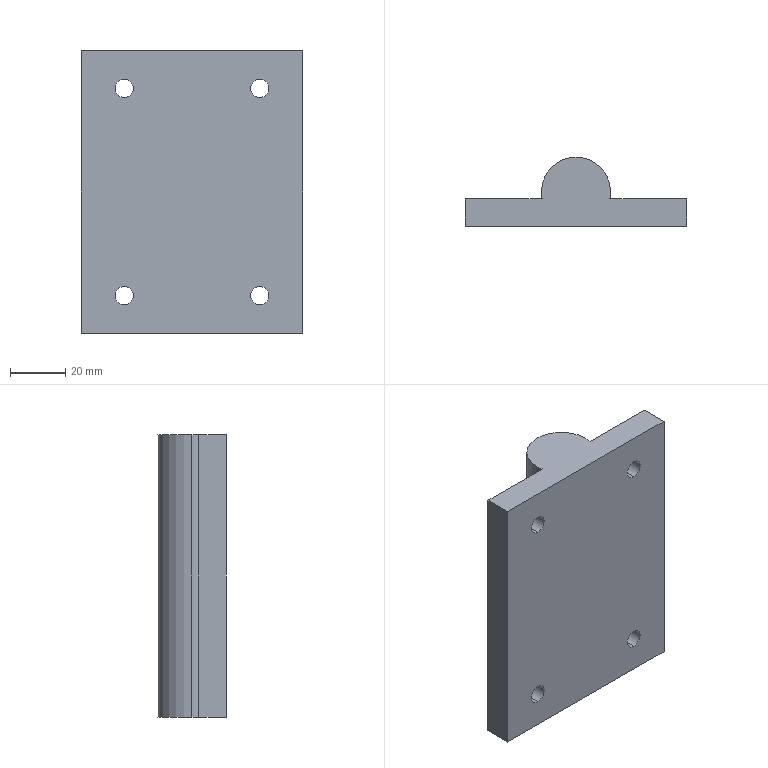Part | SolidWorks | features BaseBody 1 | 1 solid | 26 faces | box 80 x 25 x 102 mm | volume 111075 mm3 | cylinder 11 | cone 8 | plane 7 | commonest cylinder face diameters 6.6 x8 25 x3
STEP:
#1=CARTESIAN_POINT('',(-24.5,6.9,-40.8));
#2=VERTEX_POINT('',#1);
#3=CARTESIAN_POINT('',(-24.5,10.,-43.9));
#4=VERTEX_POINT('',#3);
#5=CARTESIAN_POINT('',(-24.5,10.,-43.9));
#6=DIRECTION('',(0.,0.7071,-0.7071));
#7=VECTOR('',#6,1000.);
#8=LINE('',#5,#7);
#9=EDGE_CURVE('',#2,#4,#8,.T.);
#10=ORIENTED_EDGE('',*,*,#9,.F.);
#11=CARTESIAN_POINT('',(-24.5,6.9,-34.2));
#12=VERTEX_POINT('',#11);
#13=CARTESIAN_POINT('',(-24.5,6.9,-37.5));
#14=DIRECTION('',(0.,1.,0.));
#15=DIRECTION('',(0.,0.,1.));
#16=AXIS2_PLACEMENT_3D('',#13,#14,#15);
#17=CIRCLE('',#16,3.3);
#18=EDGE_CURVE('',#12,#2,#17,.T.);
#19=ORIENTED_EDGE('',*,*,#18,.F.);
#20=CARTESIAN_POINT('',(-24.5,10.,-31.1));
#21=VERTEX_POINT('',#20);
#22=CARTESIAN_POINT('',(-24.5,10.,-31.1));
#23=DIRECTION('',(0.,0.7071,0.7071));
#24=VECTOR('',#23,1000.);
#25=LINE('',#22,#24);
#26=EDGE_CURVE('',#12,#21,#25,.T.);
#27=ORIENTED_EDGE('',*,*,#26,.T.);
#28=CARTESIAN_POINT('',(-24.5,10.,-37.5));
#29=DIRECTION('',(0.,1.,0.));
#30=DIRECTION('',(0.,0.,1.));
#31=AXIS2_PLACEMENT_3D('',#28,#29,#30);
#32=CIRCLE('',#31,6.4);
#33=EDGE_CURVE('',#21,#4,#32,.T.);
#34=ORIENTED_EDGE('',*,*,#33,.T.);
#35=EDGE_LOOP('',(#10,#19,#27,#34));
#36=FACE_OUTER_BOUND('',#35,.T.);
#37=CARTESIAN_POINT('',(-24.5,10.,-37.5));
#38=DIRECTION('',(0.,1.,0.));
#39=DIRECTION('',(0.,0.,1.));
#40=AXIS2_PLACEMENT_3D('',#37,#38,#39);
#41=CONICAL_SURFACE('',#40,6.4,0.7854);
#42=ADVANCED_FACE('',(#36),#41,.F.);
#43=CARTESIAN_POINT('',(-24.5,0.,-40.8));
#44=VERTEX_POINT('',#43);
#45=CARTESIAN_POINT('',(-24.5,10.,-40.8));
#46=DIRECTION('',(0.,1.,0.));
#47=VECTOR('',#46,1000.);
#48=LINE('',#45,#47);
#49=EDGE_CURVE('',#44,#2,#48,.T.);
#50=ORIENTED_EDGE('',*,*,#49,.F.);
#51=CARTESIAN_POINT('',(-24.5,0.,-34.2));
#52=VERTEX_POINT('',#51);
#53=CARTESIAN_POINT('',(-24.5,0.,-37.5));
#54=DIRECTION('',(0.,1.,0.));
#55=DIRECTION('',(0.,0.,1.));
#56=AXIS2_PLACEMENT_3D('',#53,#54,#55);
#57=CIRCLE('',#56,3.3);
#58=EDGE_CURVE('',#52,#44,#57,.T.);
#59=ORIENTED_EDGE('',*,*,#58,.F.);
#60=CARTESIAN_POINT('',(-24.5,10.,-34.2));
#61=DIRECTION('',(0.,1.,0.));
#62=VECTOR('',#61,1000.);
#63=LINE('',#60,#62);
#64=EDGE_CURVE('',#52,#12,#63,.T.);
#65=ORIENTED_EDGE('',*,*,#64,.T.);
#66=ORIENTED_EDGE('',*,*,#18,.T.);
#67=EDGE_LOOP('',(#50,#59,#65,#66));
#68=FACE_OUTER_BOUND('',#67,.T.);
#69=CARTESIAN_POINT('',(-24.5,10.,-37.5));
#70=DIRECTION('',(0.,1.,0.));
#71=DIRECTION('',(0.,0.,1.));
#72=AXIS2_PLACEMENT_3D('',#69,#70,#71);
#73=CYLINDRICAL_SURFACE('',#72,3.3);
#74=ADVANCED_FACE('',(#68),#73,.F.);
#75=CARTESIAN_POINT('',(-24.5,6.9,34.2));
#76=VERTEX_POINT('',#75);
#77=CARTESIAN_POINT('',(-24.5,10.,31.1));
#78=VERTEX_POINT('',#77);
#79=CARTESIAN_POINT('',(-24.5,10.,31.1));
#80=DIRECTION('',(0.,0.7071,-0.7071));
#81=VECTOR('',#80,1000.);
#82=LINE('',#79,#81);
#83=EDGE_CURVE('',#76,#78,#82,.T.);
#84=ORIENTED_EDGE('',*,*,#83,.F.);
#85=CARTESIAN_POINT('',(-24.5,6.9,40.8));
#86=VERTEX_POINT('',#85);
#87=CARTESIAN_POINT('',(-24.5,6.9,37.5));
#88=DIRECTION('',(0.,1.,0.));
#89=DIRECTION('',(0.,0.,1.));
#90=AXIS2_PLACEMENT_3D('',#87,#88,#89);
#91=CIRCLE('',#90,3.3);
#92=EDGE_CURVE('',#86,#76,#91,.T.);
#93=ORIENTED_EDGE('',*,*,#92,.F.);
#94=CARTESIAN_POINT('',(-24.5,10.,43.9));
#95=VERTEX_POINT('',#94);
#96=CARTESIAN_POINT('',(-24.5,10.,43.9));
#97=DIRECTION('',(0.,0.7071,0.7071));
#98=VECTOR('',#97,1000.);
#99=LINE('',#96,#98);
#100=EDGE_CURVE('',#86,#95,#99,.T.);
#101=ORIENTED_EDGE('',*,*,#100,.T.);
#102=CARTESIAN_POINT('',(-24.5,10.,37.5));
#103=DIRECTION('',(0.,1.,0.));
#104=DIRECTION('',(0.,0.,1.));
#105=AXIS2_PLACEMENT_3D('',#102,#103,#104);
#106=CIRCLE('',#105,6.4);
#107=EDGE_CURVE('',#95,#78,#106,.T.);
#108=ORIENTED_EDGE('',*,*,#107,.T.);
#109=EDGE_LOOP('',(#84,#93,#101,#108));
#110=FACE_OUTER_BOUND('',#109,.T.);
#111=CARTESIAN_POINT('',(-24.5,10.,37.5));
#112=DIRECTION('',(0.,1.,0.));
#113=DIRECTION('',(0.,0.,1.));
#114=AXIS2_PLACEMENT_3D('',#111,#112,#113);
#115=CONICAL_SURFACE('',#114,6.4,0.7854);
#116=ADVANCED_FACE('',(#110),#115,.F.);
#117=CARTESIAN_POINT('',(-24.5,0.,34.2));
#118=VERTEX_POINT('',#117);
#119=CARTESIAN_POINT('',(-24.5,10.,34.2));
#120=DIRECTION('',(0.,1.,0.));
#121=VECTOR('',#120,1000.);
#122=LINE('',#119,#121);
#123=EDGE_CURVE('',#118,#76,#122,.T.);
#124=ORIENTED_EDGE('',*,*,#123,.F.);
#125=CARTESIAN_POINT('',(-24.5,0.,40.8));
#126=VERTEX_POINT('',#125);
#127=CARTESIAN_POINT('',(-24.5,0.,37.5));
#128=DIRECTION('',(0.,1.,0.));
#129=DIRECTION('',(0.,0.,1.));
#130=AXIS2_PLACEMENT_3D('',#127,#128,#129);
#131=CIRCLE('',#130,3.3);
#132=EDGE_CURVE('',#126,#118,#131,.T.);
#133=ORIENTED_EDGE('',*,*,#132,.F.);
#134=CARTESIAN_POINT('',(-24.5,10.,40.8));
#135=DIRECTION('',(0.,1.,0.));
#136=VECTOR('',#135,1000.);
#137=LINE('',#134,#136);
#138=EDGE_CURVE('',#126,#86,#137,.T.);
#139=ORIENTED_EDGE('',*,*,#138,.T.);
#140=ORIENTED_EDGE('',*,*,#92,.T.);
#141=EDGE_LOOP('',(#124,#133,#139,#140));
#142=FACE_OUTER_BOUND('',#141,.T.);
#143=CARTESIAN_POINT('',(-24.5,10.,37.5));
#144=DIRECTION('',(0.,1.,0.));
#145=DIRECTION('',(0.,0.,1.));
#146=AXIS2_PLACEMENT_3D('',#143,#144,#145);
#147=CYLINDRICAL_SURFACE('',#146,3.3);
#148=ADVANCED_FACE('',(#142),#147,.F.);
#149=CARTESIAN_POINT('',(24.5,6.9,34.2));
#150=VERTEX_POINT('',#149);
#151=CARTESIAN_POINT('',(24.5,10.,31.1));
#152=VERTEX_POINT('',#151);
#153=CARTESIAN_POINT('',(24.5,10.,31.1));
#154=DIRECTION('',(0.,0.7071,-0.7071));
#155=VECTOR('',#154,1000.);
#156=LINE('',#153,#155);
#157=EDGE_CURVE('',#150,#152,#156,.T.);
#158=ORIENTED_EDGE('',*,*,#157,.F.);
#159=CARTESIAN_POINT('',(24.5,6.9,40.8));
#160=VERTEX_POINT('',#159);
#161=CARTESIAN_POINT('',(24.5,6.9,37.5));
#162=DIRECTION('',(0.,1.,0.));
#163=DIRECTION('',(0.,0.,1.));
#164=AXIS2_PLACEMENT_3D('',#161,#162,#163);
#165=CIRCLE('',#164,3.3);
#166=EDGE_CURVE('',#160,#150,#165,.T.);
#167=ORIENTED_EDGE('',*,*,#166,.F.);
#168=CARTESIAN_POINT('',(24.5,10.,43.9));
#169=VERTEX_POINT('',#168);
#170=CARTESIAN_POINT('',(24.5,10.,43.9));
#171=DIRECTION('',(0.,0.7071,0.7071));
#172=VECTOR('',#171,1000.);
#173=LINE('',#170,#172);
#174=EDGE_CURVE('',#160,#169,#173,.T.);
#175=ORIENTED_EDGE('',*,*,#174,.T.);
#176=CARTESIAN_POINT('',(24.5,10.,37.5));
#177=DIRECTION('',(0.,1.,0.));
#178=DIRECTION('',(0.,0.,1.));
#179=AXIS2_PLACEMENT_3D('',#176,#177,#178);
#180=CIRCLE('',#179,6.4);
#181=EDGE_CURVE('',#169,#152,#180,.T.);
#182=ORIENTED_EDGE('',*,*,#181,.T.);
#183=EDGE_LOOP('',(#158,#167,#175,#182));
#184=FACE_OUTER_BOUND('',#183,.T.);
#185=CARTESIAN_POINT('',(24.5,10.,37.5));
#186=DIRECTION('',(0.,1.,0.));
#187=DIRECTION('',(0.,0.,1.));
#188=AXIS2_PLACEMENT_3D('',#185,#186,#187);
#189=CONICAL_SURFACE('',#188,6.4,0.7854);
#190=ADVANCED_FACE('',(#184),#189,.F.);
#191=CARTESIAN_POINT('',(24.5,0.,34.2));
#192=VERTEX_POINT('',#191);
#193=CARTESIAN_POINT('',(24.5,10.,34.2));
#194=DIRECTION('',(0.,1.,0.));
#195=VECTOR('',#194,1000.);
#196=LINE('',#193,#195);
#197=EDGE_CURVE('',#192,#150,#196,.T.);
#198=ORIENTED_EDGE('',*,*,#197,.F.);
#199=CARTESIAN_POINT('',(24.5,0.,40.8));
#200=VERTEX_POINT('',#199);
#201=CARTESIAN_POINT('',(24.5,0.,37.5));
#202=DIRECTION('',(0.,1.,0.));
#203=DIRECTION('',(0.,0.,1.));
#204=AXIS2_PLACEMENT_3D('',#201,#202,#203);
#205=CIRCLE('',#204,3.3);
#206=EDGE_CURVE('',#200,#192,#205,.T.);
#207=ORIENTED_EDGE('',*,*,#206,.F.);
#208=CARTESIAN_POINT('',(24.5,10.,40.8));
#209=DIRECTION('',(0.,1.,0.));
#210=VECTOR('',#209,1000.);
#211=LINE('',#208,#210);
#212=EDGE_CURVE('',#200,#160,#211,.T.);
#213=ORIENTED_EDGE('',*,*,#212,.T.);
#214=ORIENTED_EDGE('',*,*,#166,.T.);
#215=EDGE_LOOP('',(#198,#207,#213,#214));
#216=FACE_OUTER_BOUND('',#215,.T.);
#217=CARTESIAN_POINT('',(24.5,10.,37.5));
#218=DIRECTION('',(0.,1.,0.));
#219=DIRECTION('',(0.,0.,1.));
#220=AXIS2_PLACEMENT_3D('',#217,#218,#219);
#221=CYLINDRICAL_SURFACE('',#220,3.3);
#222=ADVANCED_FACE('',(#216),#221,.F.);
#223=CARTESIAN_POINT('',(24.5,6.9,-40.8));
#224=VERTEX_POINT('',#223);
#225=CARTESIAN_POINT('',(24.5,10.,-43.9));
#226=VERTEX_POINT('',#225);
#227=CARTESIAN_POINT('',(24.5,10.,-43.9));
#228=DIRECTION('',(0.,0.7071,-0.7071));
#229=VECTOR('',#228,1000.);
#230=LINE('',#227,#229);
#231=EDGE_CURVE('',#224,#226,#230,.T.);
#232=ORIENTED_EDGE('',*,*,#231,.F.);
#233=CARTESIAN_POINT('',(24.5,6.9,-34.2));
#234=VERTEX_POINT('',#233);
#235=CARTESIAN_POINT('',(24.5,6.9,-37.5));
#236=DIRECTION('',(0.,1.,0.));
#237=DIRECTION('',(0.,0.,1.));
#238=AXIS2_PLACEMENT_3D('',#235,#236,#237);
#239=CIRCLE('',#238,3.3);
#240=EDGE_CURVE('',#234,#224,#239,.T.);
#241=ORIENTED_EDGE('',*,*,#240,.F.);
#242=CARTESIAN_POINT('',(24.5,10.,-31.1));
#243=VERTEX_POINT('',#242);
#244=CARTESIAN_POINT('',(24.5,10.,-31.1));
#245=DIRECTION('',(0.,0.7071,0.7071));
#246=VECTOR('',#245,1000.);
#247=LINE('',#244,#246);
#248=EDGE_CURVE('',#234,#243,#247,.T.);
#249=ORIENTED_EDGE('',*,*,#248,.T.);
#250=CARTESIAN_POINT('',(24.5,10.,-37.5));
#251=DIRECTION('',(0.,1.,0.));
#252=DIRECTION('',(0.,0.,1.));
#253=AXIS2_PLACEMENT_3D('',#250,#251,#252);
#254=CIRCLE('',#253,6.4);
#255=EDGE_CURVE('',#243,#226,#254,.T.);
#256=ORIENTED_EDGE('',*,*,#255,.T.);
#257=EDGE_LOOP('',(#232,#241,#249,#256));
#258=FACE_OUTER_BOUND('',#257,.T.);
#259=CARTESIAN_POINT('',(24.5,10.,-37.5));
#260=DIRECTION('',(0.,1.,0.));
#261=DIRECTION('',(0.,0.,1.));
#262=AXIS2_PLACEMENT_3D('',#259,#260,#261);
#263=CONICAL_SURFACE('',#262,6.4,0.7854);
#264=ADVANCED_FACE('',(#258),#263,.F.);
#265=CARTESIAN_POINT('',(24.5,0.,-40.8));
#266=VERTEX_POINT('',#265);
#267=CARTESIAN_POINT('',(24.5,10.,-40.8));
#268=DIRECTION('',(0.,1.,0.));
#269=VECTOR('',#268,1000.);
#270=LINE('',#267,#269);
#271=EDGE_CURVE('',#266,#224,#270,.T.);
#272=ORIENTED_EDGE('',*,*,#271,.F.);
#273=CARTESIAN_POINT('',(24.5,0.,-34.2));
#274=VERTEX_POINT('',#273);
#275=CARTESIAN_POINT('',(24.5,0.,-37.5));
#276=DIRECTION('',(0.,1.,0.));
#277=DIRECTION('',(0.,0.,1.));
#278=AXIS2_PLACEMENT_3D('',#275,#276,#277);
#279=CIRCLE('',#278,3.3);
#280=EDGE_CURVE('',#274,#266,#279,.T.);
#281=ORIENTED_EDGE('',*,*,#280,.F.);
#282=CARTESIAN_POINT('',(24.5,10.,-34.2));
#283=DIRECTION('',(0.,1.,0.));
#284=VECTOR('',#283,1000.);
#285=LINE('',#282,#284);
#286=EDGE_CURVE('',#274,#234,#285,.T.);
#287=ORIENTED_EDGE('',*,*,#286,.T.);
#288=ORIENTED_EDGE('',*,*,#240,.T.);
#289=EDGE_LOOP('',(#272,#281,#287,#288));
#290=FACE_OUTER_BOUND('',#289,.T.);
#291=CARTESIAN_POINT('',(24.5,10.,-37.5));
#292=DIRECTION('',(0.,1.,0.));
#293=DIRECTION('',(0.,0.,1.));
#294=AXIS2_PLACEMENT_3D('',#291,#292,#293);
#295=CYLINDRICAL_SURFACE('',#294,3.3);
#296=ADVANCED_FACE('',(#290),#295,.F.);
#297=CARTESIAN_POINT('',(12.5,12.5,51.));
#298=VERTEX_POINT('',#297);
#299=CARTESIAN_POINT('',(12.5,12.5,-51.));
#300=VERTEX_POINT('',#299);
#301=CARTESIAN_POINT('',(12.5,12.5,51.));
#302=DIRECTION('',(0.,0.,-1.));
#303=VECTOR('',#302,1000.);
#304=LINE('',#301,#303);
#305=EDGE_CURVE('',#298,#300,#304,.T.);
#306=ORIENTED_EDGE('',*,*,#305,.F.);
#307=CARTESIAN_POINT('',(12.247,10.,51.));
#308=VERTEX_POINT('',#307);
#309=CARTESIAN_POINT('',(0.,12.5,51.));
#310=DIRECTION('',(0.,0.,1.));
#311=DIRECTION('',(1.,0.,0.));
#312=AXIS2_PLACEMENT_3D('',#309,#310,#311);
#313=CIRCLE('',#312,12.5);
#314=EDGE_CURVE('',#308,#298,#313,.T.);
#315=ORIENTED_EDGE('',*,*,#314,.F.);
#316=CARTESIAN_POINT('',(12.247,10.,-51.));
#317=VERTEX_POINT('',#316);
#318=CARTESIAN_POINT('',(12.247,10.,51.));
#319=DIRECTION('',(0.,0.,1.));
#320=VECTOR('',#319,1000.);
#321=LINE('',#318,#320);
#322=EDGE_CURVE('',#317,#308,#321,.T.);
#323=ORIENTED_EDGE('',*,*,#322,.F.);
#324=CARTESIAN_POINT('',(0.,12.5,-51.));
#325=DIRECTION('',(0.,0.,1.));
#326=DIRECTION('',(1.,0.,0.));
#327=AXIS2_PLACEMENT_3D('',#324,#325,#326);
#328=CIRCLE('',#327,12.5);
#329=EDGE_CURVE('',#317,#300,#328,.T.);
#330=ORIENTED_EDGE('',*,*,#329,.T.);
#331=EDGE_LOOP('',(#306,#315,#323,#330));
#332=FACE_OUTER_BOUND('',#331,.T.);
#333=CARTESIAN_POINT('',(0.,12.5,51.));
#334=DIRECTION('',(0.,0.,-1.));
#335=DIRECTION('',(-1.,0.,0.));
#336=AXIS2_PLACEMENT_3D('',#333,#334,#335);
#337=CYLINDRICAL_SURFACE('',#336,12.5);
#338=ADVANCED_FACE('',(#332),#337,.T.);
#339=ORIENTED_EDGE('',*,*,#280,.T.);
#340=CARTESIAN_POINT('',(24.5,0.,-37.5));
#341=DIRECTION('',(0.,1.,0.));
#342=DIRECTION('',(0.,0.,1.));
#343=AXIS2_PLACEMENT_3D('',#340,#341,#342);
#344=CIRCLE('',#343,3.3);
#345=EDGE_CURVE('',#266,#274,#344,.T.);
#346=ORIENTED_EDGE('',*,*,#345,.T.);
#347=EDGE_LOOP('',(#339,#346));
#348=FACE_BOUND('',#347,.T.);
#349=ORIENTED_EDGE('',*,*,#206,.T.);
#350=CARTESIAN_POINT('',(24.5,0.,37.5));
#351=DIRECTION('',(0.,1.,0.));
#352=DIRECTION('',(0.,0.,1.));
#353=AXIS2_PLACEMENT_3D('',#350,#351,#352);
#354=CIRCLE('',#353,3.3);
#355=EDGE_CURVE('',#192,#200,#354,.T.);
#356=ORIENTED_EDGE('',*,*,#355,.T.);
#357=EDGE_LOOP('',(#349,#356));
#358=FACE_BOUND('',#357,.T.);
#359=ORIENTED_EDGE('',*,*,#132,.T.);
#360=CARTESIAN_POINT('',(-24.5,0.,37.5));
#361=DIRECTION('',(0.,1.,0.));
#362=DIRECTION('',(0.,0.,1.));
#363=AXIS2_PLACEMENT_3D('',#360,#361,#362);
#364=CIRCLE('',#363,3.3);
#365=EDGE_CURVE('',#118,#126,#364,.T.);
#366=ORIENTED_EDGE('',*,*,#365,.T.);
#367=EDGE_LOOP('',(#359,#366));
#368=FACE_BOUND('',#367,.T.);
#369=ORIENTED_EDGE('',*,*,#58,.T.);
#370=CARTESIAN_POINT('',(-24.5,0.,-37.5));
#371=DIRECTION('',(0.,1.,0.));
#372=DIRECTION('',(0.,0.,1.));
#373=AXIS2_PLACEMENT_3D('',#370,#371,#372);
#374=CIRCLE('',#373,3.3);
#375=EDGE_CURVE('',#44,#52,#374,.T.);
#376=ORIENTED_EDGE('',*,*,#375,.T.);
#377=EDGE_LOOP('',(#369,#376));
#378=FACE_BOUND('',#377,.T.);
#379=CARTESIAN_POINT('',(-40.,0.,-51.));
#380=VERTEX_POINT('',#379);
#381=CARTESIAN_POINT('',(-40.,0.,51.));
#382=VERTEX_POINT('',#381);
#383=CARTESIAN_POINT('',(-40.,0.,-51.));
#384=DIRECTION('',(0.,0.,1.));
#385=VECTOR('',#384,1000.);
#386=LINE('',#383,#385);
#387=EDGE_CURVE('',#380,#382,#386,.T.);
#388=ORIENTED_EDGE('',*,*,#387,.F.);
#389=CARTESIAN_POINT('',(40.,0.,-51.));
#390=VERTEX_POINT('',#389);
#391=CARTESIAN_POINT('',(-40.,0.,-51.));
#392=DIRECTION('',(-1.,0.,0.));
#393=VECTOR('',#392,1000.);
#394=LINE('',#391,#393);
#395=EDGE_CURVE('',#390,#380,#394,.T.);
#396=ORIENTED_EDGE('',*,*,#395,.F.);
#397=CARTESIAN_POINT('',(40.,0.,51.));
#398=VERTEX_POINT('',#397);
#399=CARTESIAN_POINT('',(40.,0.,-51.));
#400=DIRECTION('',(0.,0.,-1.));
#401=VECTOR('',#400,1000.);
#402=LINE('',#399,#401);
#403=EDGE_CURVE('',#398,#390,#402,.T.);
#404=ORIENTED_EDGE('',*,*,#403,.F.);
#405=CARTESIAN_POINT('',(-40.,0.,51.));
#406=DIRECTION('',(1.,0.,0.));
#407=VECTOR('',#406,1000.);
#408=LINE('',#405,#407);
#409=EDGE_CURVE('',#382,#398,#408,.T.);
#410=ORIENTED_EDGE('',*,*,#409,.F.);
#411=EDGE_LOOP('',(#388,#396,#404,#410));
#412=FACE_OUTER_BOUND('',#411,.T.);
#413=CARTESIAN_POINT('',(0.,0.,0.));
#414=DIRECTION('',(0.,1.,0.));
#415=DIRECTION('',(1.,0.,0.));
#416=AXIS2_PLACEMENT_3D('',#413,#414,#415);
#417=PLANE('',#416);
#418=ADVANCED_FACE('',(#348,#358,#368,#378,#412),#417,.F.);
#419=CARTESIAN_POINT('',(40.,10.,51.));
#420=VERTEX_POINT('',#419);
#421=CARTESIAN_POINT('',(-40.,10.,51.));
#422=DIRECTION('',(1.,0.,0.));
#423=VECTOR('',#422,1000.);
#424=LINE('',#421,#423);
#425=EDGE_CURVE('',#308,#420,#424,.T.);
#426=ORIENTED_EDGE('',*,*,#425,.F.);
#427=ORIENTED_EDGE('',*,*,#314,.T.);
#428=CARTESIAN_POINT('',(-12.5,12.5,51.));
#429=VERTEX_POINT('',#428);
#430=CARTESIAN_POINT('',(0.,12.5,51.));
#431=DIRECTION('',(0.,0.,1.));
#432=DIRECTION('',(1.,0.,0.));
#433=AXIS2_PLACEMENT_3D('',#430,#431,#432);
#434=CIRCLE('',#433,12.5);
#435=EDGE_CURVE('',#298,#429,#434,.T.);
#436=ORIENTED_EDGE('',*,*,#435,.T.);
#437=CARTESIAN_POINT('',(-12.247,10.,51.));
#438=VERTEX_POINT('',#437);
#439=CARTESIAN_POINT('',(0.,12.5,51.));
#440=DIRECTION('',(0.,0.,1.));
#441=DIRECTION('',(1.,0.,0.));
#442=AXIS2_PLACEMENT_3D('',#439,#440,#441);
#443=CIRCLE('',#442,12.5);
#444=EDGE_CURVE('',#429,#438,#443,.T.);
#445=ORIENTED_EDGE('',*,*,#444,.T.);
#446=CARTESIAN_POINT('',(-40.,10.,51.));
#447=VERTEX_POINT('',#446);
#448=CARTESIAN_POINT('',(-40.,10.,51.));
#449=DIRECTION('',(1.,0.,0.));
#450=VECTOR('',#449,1000.);
#451=LINE('',#448,#450);
#452=EDGE_CURVE('',#447,#438,#451,.T.);
#453=ORIENTED_EDGE('',*,*,#452,.F.);
#454=CARTESIAN_POINT('',(-40.,10.,51.));
#455=DIRECTION('',(0.,-1.,0.));
#456=VECTOR('',#455,1000.);
#457=LINE('',#454,#456);
#458=EDGE_CURVE('',#447,#382,#457,.T.);
#459=ORIENTED_EDGE('',*,*,#458,.T.);
#460=ORIENTED_EDGE('',*,*,#409,.T.);
#461=CARTESIAN_POINT('',(40.,10.,51.));
#462=DIRECTION('',(0.,-1.,0.));
#463=VECTOR('',#462,1000.);
#464=LINE('',#461,#463);
#465=EDGE_CURVE('',#420,#398,#464,.T.);
#466=ORIENTED_EDGE('',*,*,#465,.F.);
#467=EDGE_LOOP('',(#426,#427,#436,#445,#453,#459,#460,#466));
#468=FACE_OUTER_BOUND('',#467,.T.);
#469=CARTESIAN_POINT('',(-40.,10.,51.));
#470=DIRECTION('',(0.,0.,-1.));
#471=DIRECTION('',(0.,-1.,0.));
#472=AXIS2_PLACEMENT_3D('',#469,#470,#471);
#473=PLANE('',#472);
#474=ADVANCED_FACE('',(#468),#473,.F.);
#475=ORIENTED_EDGE('',*,*,#387,.T.);
#476=ORIENTED_EDGE('',*,*,#458,.F.);
#477=CARTESIAN_POINT('',(-40.,10.,-51.));
#478=VERTEX_POINT('',#477);
#479=CARTESIAN_POINT('',(-40.,10.,-51.));
#480=DIRECTION('',(0.,0.,1.));
#481=VECTOR('',#480,1000.);
#482=LINE('',#479,#481);
#483=EDGE_CURVE('',#478,#447,#482,.T.);
#484=ORIENTED_EDGE('',*,*,#483,.F.);
#485=CARTESIAN_POINT('',(-40.,10.,-51.));
#486=DIRECTION('',(0.,-1.,0.));
#487=VECTOR('',#486,1000.);
#488=LINE('',#485,#487);
#489=EDGE_CURVE('',#478,#380,#488,.T.);
#490=ORIENTED_EDGE('',*,*,#489,.T.);
#491=EDGE_LOOP('',(#475,#476,#484,#490));
#492=FACE_OUTER_BOUND('',#491,.T.);
#493=CARTESIAN_POINT('',(-40.,10.,-51.));
#494=DIRECTION('',(1.,0.,0.));
#495=DIRECTION('',(0.,0.,-1.));
#496=AXIS2_PLACEMENT_3D('',#493,#494,#495);
#497=PLANE('',#496);
#498=ADVANCED_FACE('',(#492),#497,.F.);
#499=CARTESIAN_POINT('',(-12.247,10.,-51.));
#500=VERTEX_POINT('',#499);
#501=CARTESIAN_POINT('',(-40.,10.,-51.));
#502=DIRECTION('',(-1.,0.,0.));
#503=VECTOR('',#502,1000.);
#504=LINE('',#501,#503);
#505=EDGE_CURVE('',#500,#478,#504,.T.);
#506=ORIENTED_EDGE('',*,*,#505,.F.);
#507=CARTESIAN_POINT('',(-12.5,12.5,-51.));
#508=VERTEX_POINT('',#507);
#509=CARTESIAN_POINT('',(0.,12.5,-51.));
#510=DIRECTION('',(0.,0.,1.));
#511=DIRECTION('',(1.,0.,0.));
#512=AXIS2_PLACEMENT_3D('',#509,#510,#511);
#513=CIRCLE('',#512,12.5);
#514=EDGE_CURVE('',#508,#500,#513,.T.);
#515=ORIENTED_EDGE('',*,*,#514,.F.);
#516=CARTESIAN_POINT('',(0.,12.5,-51.));
#517=DIRECTION('',(0.,0.,1.));
#518=DIRECTION('',(1.,0.,0.));
#519=AXIS2_PLACEMENT_3D('',#516,#517,#518);
#520=CIRCLE('',#519,12.5);
#521=EDGE_CURVE('',#300,#508,#520,.T.);
#522=ORIENTED_EDGE('',*,*,#521,.F.);
#523=ORIENTED_EDGE('',*,*,#329,.F.);
#524=CARTESIAN_POINT('',(40.,10.,-51.));
#525=VERTEX_POINT('',#524);
#526=CARTESIAN_POINT('',(-40.,10.,-51.));
#527=DIRECTION('',(-1.,0.,0.));
#528=VECTOR('',#527,1000.);
#529=LINE('',#526,#528);
#530=EDGE_CURVE('',#525,#317,#529,.T.);
#531=ORIENTED_EDGE('',*,*,#530,.F.);
#532=CARTESIAN_POINT('',(40.,10.,-51.));
#533=DIRECTION('',(0.,-1.,0.));
#534=VECTOR('',#533,1000.);
#535=LINE('',#532,#534);
#536=EDGE_CURVE('',#525,#390,#535,.T.);
#537=ORIENTED_EDGE('',*,*,#536,.T.);
#538=ORIENTED_EDGE('',*,*,#395,.T.);
#539=ORIENTED_EDGE('',*,*,#489,.F.);
#540=EDGE_LOOP('',(#506,#515,#522,#523,#531,#537,#538,#539));
#541=FACE_OUTER_BOUND('',#540,.T.);
#542=CARTESIAN_POINT('',(-40.,10.,-51.));
#543=DIRECTION('',(0.,0.,1.));
#544=DIRECTION('',(1.,0.,0.));
#545=AXIS2_PLACEMENT_3D('',#542,#543,#544);
#546=PLANE('',#545);
#547=ADVANCED_FACE('',(#541),#546,.F.);
#548=ORIENTED_EDGE('',*,*,#403,.T.);
#549=ORIENTED_EDGE('',*,*,#536,.F.);
#550=CARTESIAN_POINT('',(40.,10.,-51.));
#551=DIRECTION('',(0.,0.,-1.));
#552=VECTOR('',#551,1000.);
#553=LINE('',#550,#552);
#554=EDGE_CURVE('',#420,#525,#553,.T.);
#555=ORIENTED_EDGE('',*,*,#554,.F.);
#556=ORIENTED_EDGE('',*,*,#465,.T.);
#557=EDGE_LOOP('',(#548,#549,#555,#556));
#558=FACE_OUTER_BOUND('',#557,.T.);
#559=CARTESIAN_POINT('',(40.,10.,-51.));
#560=DIRECTION('',(-1.,0.,0.));
#561=DIRECTION('',(0.,1.,0.));
#562=AXIS2_PLACEMENT_3D('',#559,#560,#561);
#563=PLANE('',#562);
#564=ADVANCED_FACE('',(#558),#563,.F.);
#565=ORIENTED_EDGE('',*,*,#107,.F.);
#566=CARTESIAN_POINT('',(-24.5,10.,37.5));
#567=DIRECTION('',(0.,1.,0.));
#568=DIRECTION('',(0.,0.,1.));
#569=AXIS2_PLACEMENT_3D('',#566,#567,#568);
#570=CIRCLE('',#569,6.4);
#571=EDGE_CURVE('',#78,#95,#570,.T.);
#572=ORIENTED_EDGE('',*,*,#571,.F.);
#573=EDGE_LOOP('',(#565,#572));
#574=FACE_BOUND('',#573,.T.);
#575=ORIENTED_EDGE('',*,*,#33,.F.);
#576=CARTESIAN_POINT('',(-24.5,10.,-37.5));
#577=DIRECTION('',(0.,1.,0.));
#578=DIRECTION('',(0.,0.,1.));
#579=AXIS2_PLACEMENT_3D('',#576,#577,#578);
#580=CIRCLE('',#579,6.4);
#581=EDGE_CURVE('',#4,#21,#580,.T.);
#582=ORIENTED_EDGE('',*,*,#581,.F.);
#583=EDGE_LOOP('',(#575,#582));
#584=FACE_BOUND('',#583,.T.);
#585=ORIENTED_EDGE('',*,*,#452,.T.);
#586=CARTESIAN_POINT('',(-12.247,10.,51.));
#587=DIRECTION('',(0.,0.,-1.));
#588=VECTOR('',#587,1000.);
#589=LINE('',#586,#588);
#590=EDGE_CURVE('',#438,#500,#589,.T.);
#591=ORIENTED_EDGE('',*,*,#590,.T.);
#592=ORIENTED_EDGE('',*,*,#505,.T.);
#593=ORIENTED_EDGE('',*,*,#483,.T.);
#594=EDGE_LOOP('',(#585,#591,#592,#593));
#595=FACE_OUTER_BOUND('',#594,.T.);
#596=CARTESIAN_POINT('',(0.,10.,0.));
#597=DIRECTION('',(0.,1.,0.));
#598=DIRECTION('',(1.,0.,0.));
#599=AXIS2_PLACEMENT_3D('',#596,#597,#598);
#600=PLANE('',#599);
#601=ADVANCED_FACE('',(#574,#584,#595),#600,.T.);
#602=ORIENTED_EDGE('',*,*,#255,.F.);
#603=CARTESIAN_POINT('',(24.5,10.,-37.5));
#604=DIRECTION('',(0.,1.,0.));
#605=DIRECTION('',(0.,0.,1.));
#606=AXIS2_PLACEMENT_3D('',#603,#604,#605);
#607=CIRCLE('',#606,6.4);
#608=EDGE_CURVE('',#226,#243,#607,.T.);
#609=ORIENTED_EDGE('',*,*,#608,.F.);
#610=EDGE_LOOP('',(#602,#609));
#611=FACE_BOUND('',#610,.T.);
#612=ORIENTED_EDGE('',*,*,#181,.F.);
#613=CARTESIAN_POINT('',(24.5,10.,37.5));
#614=DIRECTION('',(0.,1.,0.));
#615=DIRECTION('',(0.,0.,1.));
#616=AXIS2_PLACEMENT_3D('',#613,#614,#615);
#617=CIRCLE('',#616,6.4);
#618=EDGE_CURVE('',#152,#169,#617,.T.);
#619=ORIENTED_EDGE('',*,*,#618,.F.);
#620=EDGE_LOOP('',(#612,#619));
#621=FACE_BOUND('',#620,.T.);
#622=ORIENTED_EDGE('',*,*,#530,.T.);
#623=ORIENTED_EDGE('',*,*,#322,.T.);
#624=ORIENTED_EDGE('',*,*,#425,.T.);
#625=ORIENTED_EDGE('',*,*,#554,.T.);
#626=EDGE_LOOP('',(#622,#623,#624,#625));
#627=FACE_OUTER_BOUND('',#626,.T.);
#628=CARTESIAN_POINT('',(0.,10.,0.));
#629=DIRECTION('',(0.,1.,0.));
#630=DIRECTION('',(1.,0.,0.));
#631=AXIS2_PLACEMENT_3D('',#628,#629,#630);
#632=PLANE('',#631);
#633=ADVANCED_FACE('',(#611,#621,#627),#632,.T.);
#634=ORIENTED_EDGE('',*,*,#444,.F.);
#635=CARTESIAN_POINT('',(-12.5,12.5,51.));
#636=DIRECTION('',(0.,0.,-1.));
#637=VECTOR('',#636,1000.);
#638=LINE('',#635,#637);
#639=EDGE_CURVE('',#429,#508,#638,.T.);
#640=ORIENTED_EDGE('',*,*,#639,.T.);
#641=ORIENTED_EDGE('',*,*,#514,.T.);
#642=ORIENTED_EDGE('',*,*,#590,.F.);
#643=EDGE_LOOP('',(#634,#640,#641,#642));
#644=FACE_OUTER_BOUND('',#643,.T.);
#645=CARTESIAN_POINT('',(0.,12.5,51.));
#646=DIRECTION('',(0.,0.,-1.));
#647=DIRECTION('',(-1.,0.,0.));
#648=AXIS2_PLACEMENT_3D('',#645,#646,#647);
#649=CYLINDRICAL_SURFACE('',#648,12.5);
#650=ADVANCED_FACE('',(#644),#649,.T.);
#651=ORIENTED_EDGE('',*,*,#435,.F.);
#652=ORIENTED_EDGE('',*,*,#305,.T.);
#653=ORIENTED_EDGE('',*,*,#521,.T.);
#654=ORIENTED_EDGE('',*,*,#639,.F.);
#655=EDGE_LOOP('',(#651,#652,#653,#654));
#656=FACE_OUTER_BOUND('',#655,.T.);
#657=CARTESIAN_POINT('',(0.,12.5,51.));
#658=DIRECTION('',(0.,0.,-1.));
#659=DIRECTION('',(-1.,0.,0.));
#660=AXIS2_PLACEMENT_3D('',#657,#658,#659);
#661=CYLINDRICAL_SURFACE('',#660,12.5);
#662=ADVANCED_FACE('',(#656),#661,.T.);
#663=ORIENTED_EDGE('',*,*,#345,.F.);
#664=ORIENTED_EDGE('',*,*,#271,.T.);
#665=CARTESIAN_POINT('',(24.5,6.9,-37.5));
#666=DIRECTION('',(0.,1.,0.));
#667=DIRECTION('',(0.,0.,1.));
#668=AXIS2_PLACEMENT_3D('',#665,#666,#667);
#669=CIRCLE('',#668,3.3);
#670=EDGE_CURVE('',#224,#234,#669,.T.);
#671=ORIENTED_EDGE('',*,*,#670,.T.);
#672=ORIENTED_EDGE('',*,*,#286,.F.);
#673=EDGE_LOOP('',(#663,#664,#671,#672));
#674=FACE_OUTER_BOUND('',#673,.T.);
#675=CARTESIAN_POINT('',(24.5,10.,-37.5));
#676=DIRECTION('',(0.,1.,0.));
#677=DIRECTION('',(0.,0.,1.));
#678=AXIS2_PLACEMENT_3D('',#675,#676,#677);
#679=CYLINDRICAL_SURFACE('',#678,3.3);
#680=ADVANCED_FACE('',(#674),#679,.F.);
#681=ORIENTED_EDGE('',*,*,#670,.F.);
#682=ORIENTED_EDGE('',*,*,#231,.T.);
#683=ORIENTED_EDGE('',*,*,#608,.T.);
#684=ORIENTED_EDGE('',*,*,#248,.F.);
#685=EDGE_LOOP('',(#681,#682,#683,#684));
#686=FACE_OUTER_BOUND('',#685,.T.);
#687=CARTESIAN_POINT('',(24.5,10.,-37.5));
#688=DIRECTION('',(0.,1.,0.));
#689=DIRECTION('',(0.,0.,1.));
#690=AXIS2_PLACEMENT_3D('',#687,#688,#689);
#691=CONICAL_SURFACE('',#690,6.4,0.7854);
#692=ADVANCED_FACE('',(#686),#691,.F.);
#693=ORIENTED_EDGE('',*,*,#355,.F.);
#694=ORIENTED_EDGE('',*,*,#197,.T.);
#695=CARTESIAN_POINT('',(24.5,6.9,37.5));
#696=DIRECTION('',(0.,1.,0.));
#697=DIRECTION('',(0.,0.,1.));
#698=AXIS2_PLACEMENT_3D('',#695,#696,#697);
#699=CIRCLE('',#698,3.3);
#700=EDGE_CURVE('',#150,#160,#699,.T.);
#701=ORIENTED_EDGE('',*,*,#700,.T.);
#702=ORIENTED_EDGE('',*,*,#212,.F.);
#703=EDGE_LOOP('',(#693,#694,#701,#702));
#704=FACE_OUTER_BOUND('',#703,.T.);
#705=CARTESIAN_POINT('',(24.5,10.,37.5));
#706=DIRECTION('',(0.,1.,0.));
#707=DIRECTION('',(0.,0.,1.));
#708=AXIS2_PLACEMENT_3D('',#705,#706,#707);
#709=CYLINDRICAL_SURFACE('',#708,3.3);
#710=ADVANCED_FACE('',(#704),#709,.F.);
#711=ORIENTED_EDGE('',*,*,#700,.F.);
#712=ORIENTED_EDGE('',*,*,#157,.T.);
#713=ORIENTED_EDGE('',*,*,#618,.T.);
#714=ORIENTED_EDGE('',*,*,#174,.F.);
#715=EDGE_LOOP('',(#711,#712,#713,#714));
#716=FACE_OUTER_BOUND('',#715,.T.);
#717=CARTESIAN_POINT('',(24.5,10.,37.5));
#718=DIRECTION('',(0.,1.,0.));
#719=DIRECTION('',(0.,0.,1.));
#720=AXIS2_PLACEMENT_3D('',#717,#718,#719);
#721=CONICAL_SURFACE('',#720,6.4,0.7854);
#722=ADVANCED_FACE('',(#716),#721,.F.);
#723=ORIENTED_EDGE('',*,*,#365,.F.);
#724=ORIENTED_EDGE('',*,*,#123,.T.);
#725=CARTESIAN_POINT('',(-24.5,6.9,37.5));
#726=DIRECTION('',(0.,1.,0.));
#727=DIRECTION('',(0.,0.,1.));
#728=AXIS2_PLACEMENT_3D('',#725,#726,#727);
#729=CIRCLE('',#728,3.3);
#730=EDGE_CURVE('',#76,#86,#729,.T.);
#731=ORIENTED_EDGE('',*,*,#730,.T.);
#732=ORIENTED_EDGE('',*,*,#138,.F.);
#733=EDGE_LOOP('',(#723,#724,#731,#732));
#734=FACE_OUTER_BOUND('',#733,.T.);
#735=CARTESIAN_POINT('',(-24.5,10.,37.5));
#736=DIRECTION('',(0.,1.,0.));
#737=DIRECTION('',(0.,0.,1.));
#738=AXIS2_PLACEMENT_3D('',#735,#736,#737);
#739=CYLINDRICAL_SURFACE('',#738,3.3);
#740=ADVANCED_FACE('',(#734),#739,.F.);
#741=ORIENTED_EDGE('',*,*,#730,.F.);
#742=ORIENTED_EDGE('',*,*,#83,.T.);
#743=ORIENTED_EDGE('',*,*,#571,.T.);
#744=ORIENTED_EDGE('',*,*,#100,.F.);
#745=EDGE_LOOP('',(#741,#742,#743,#744));
#746=FACE_OUTER_BOUND('',#745,.T.);
#747=CARTESIAN_POINT('',(-24.5,10.,37.5));
#748=DIRECTION('',(0.,1.,0.));
#749=DIRECTION('',(0.,0.,1.));
#750=AXIS2_PLACEMENT_3D('',#747,#748,#749);
#751=CONICAL_SURFACE('',#750,6.4,0.7854);
#752=ADVANCED_FACE('',(#746),#751,.F.);
#753=ORIENTED_EDGE('',*,*,#375,.F.);
#754=ORIENTED_EDGE('',*,*,#49,.T.);
#755=CARTESIAN_POINT('',(-24.5,6.9,-37.5));
#756=DIRECTION('',(0.,1.,0.));
#757=DIRECTION('',(0.,0.,1.));
#758=AXIS2_PLACEMENT_3D('',#755,#756,#757);
#759=CIRCLE('',#758,3.3);
#760=EDGE_CURVE('',#2,#12,#759,.T.);
#761=ORIENTED_EDGE('',*,*,#760,.T.);
#762=ORIENTED_EDGE('',*,*,#64,.F.);
#763=EDGE_LOOP('',(#753,#754,#761,#762));
#764=FACE_OUTER_BOUND('',#763,.T.);
#765=CARTESIAN_POINT('',(-24.5,10.,-37.5));
#766=DIRECTION('',(0.,1.,0.));
#767=DIRECTION('',(0.,0.,1.));
#768=AXIS2_PLACEMENT_3D('',#765,#766,#767);
#769=CYLINDRICAL_SURFACE('',#768,3.3);
#770=ADVANCED_FACE('',(#764),#769,.F.);
#771=ORIENTED_EDGE('',*,*,#760,.F.);
#772=ORIENTED_EDGE('',*,*,#9,.T.);
#773=ORIENTED_EDGE('',*,*,#581,.T.);
#774=ORIENTED_EDGE('',*,*,#26,.F.);
#775=EDGE_LOOP('',(#771,#772,#773,#774));
#776=FACE_OUTER_BOUND('',#775,.T.);
#777=CARTESIAN_POINT('',(-24.5,10.,-37.5));
#778=DIRECTION('',(0.,1.,0.));
#779=DIRECTION('',(0.,0.,1.));
#780=AXIS2_PLACEMENT_3D('',#777,#778,#779);
#781=CONICAL_SURFACE('',#780,6.4,0.7854);
#782=ADVANCED_FACE('',(#776),#781,.F.);
#783=CLOSED_SHELL('',(#42,#74,#116,#148,#190,#222,#264,#296,#338,#418,#474,#498,#547,#564,#601,#633,#650,#662,#680,#692,#710,#722,#740,#752,#770,#782));
#784=MANIFOLD_SOLID_BREP('',#783);
#785=CARTESIAN_POINT('',(0.,0.,0.));
#786=DIRECTION('',(0.,0.,1.));
#787=DIRECTION('',(1.,0.,0.));
#788=AXIS2_PLACEMENT_3D('',#785,#786,#787);
#789=(LENGTH_UNIT()NAMED_UNIT(*)SI_UNIT(.MILLI.,.METRE.));
#790=UNCERTAINTY_MEASURE_WITH_UNIT(LENGTH_MEASURE(0.00001),#789,'','');
#791=(NAMED_UNIT(*)PLANE_ANGLE_UNIT()SI_UNIT($,.RADIAN.));
#792=(NAMED_UNIT(*)SI_UNIT($,.STERADIAN.)SOLID_ANGLE_UNIT());
#793=(GEOMETRIC_REPRESENTATION_CONTEXT(3)GLOBAL_UNCERTAINTY_ASSIGNED_CONTEXT((#790))GLOBAL_UNIT_ASSIGNED_CONTEXT((#789,#791,#792))REPRESENTATION_CONTEXT('',''));
#794=ADVANCED_BREP_SHAPE_REPRESENTATION('',(#784,#788),#793);